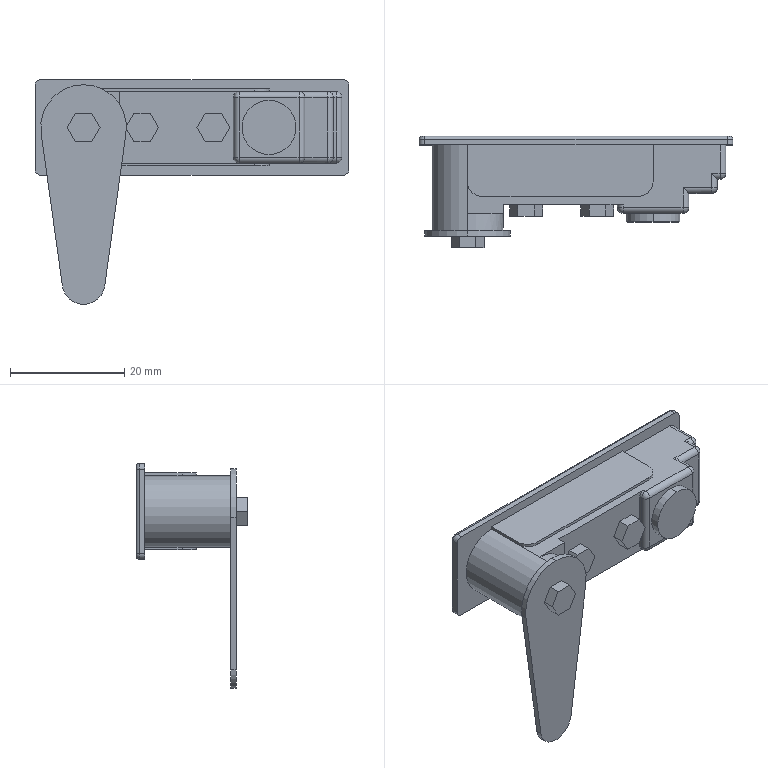Part | SolidWorks | features ICE 11, Fillet 7, BossThin 2, CutThin 2, LPattern 2, CirPattern 1, Emboss 1, Extrusion 1, MirrorPattern 1, Scale 1 | 1 solid | 237 faces | box 55 x 19.5 x 39.375 mm | volume 9114 mm3 | plane 120 | cylinder 69 | spline 28 | torus 12 | sphere 8 | commonest cylinder face diameters 2 x24 0.5 x8 0.75 x8 1 x6 5 x5 7.5 x3